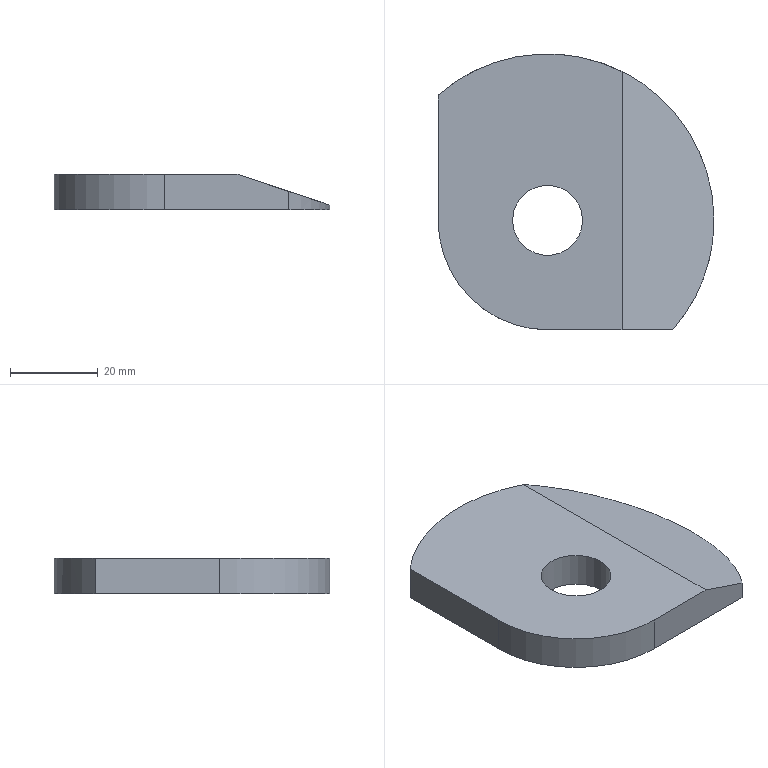Part | NX | features DATUM_CSYS 3, EXTRUDE 2, SKETCH 2 | 1 solid | 10 faces | box 62.986 x 63 x 8 mm | volume 22550 mm3 | plane 6 | cylinder 4 | commonest cylinder face diameters 76 x2 16 x1 50 x1
STEP:
#1=CARTESIAN_POINT('',(17.001,-24.999,8.));
#2=VERTEX_POINT('',#1);
#3=CARTESIAN_POINT('',(28.619,-24.999,4.125));
#4=VERTEX_POINT('',#3);
#5=CARTESIAN_POINT('',(1.895,-24.999,13.039));
#6=DIRECTION('',(0.9486,0.,-0.3164));
#7=VECTOR('',#6,1000.);
#8=LINE('',#5,#7);
#9=EDGE_CURVE('',#2,#4,#8,.T.);
#10=ORIENTED_EDGE('',*,*,#9,.F.);
#11=CARTESIAN_POINT('',(0.2147,-24.999,8.));
#12=VERTEX_POINT('',#11);
#13=CARTESIAN_POINT('',(0.2147,-24.999,8.));
#14=DIRECTION('',(1.,0.,0.));
#15=VECTOR('',#14,1000.);
#16=LINE('',#13,#15);
#17=EDGE_CURVE('',#12,#2,#16,.T.);
#18=ORIENTED_EDGE('',*,*,#17,.F.);
#19=CARTESIAN_POINT('',(0.2147,-24.999,0.));
#20=VERTEX_POINT('',#19);
#21=CARTESIAN_POINT('',(0.2147,-24.999,8.));
#22=DIRECTION('',(0.,0.,-1.));
#23=VECTOR('',#22,1000.);
#24=LINE('',#21,#23);
#25=EDGE_CURVE('',#12,#20,#24,.T.);
#26=ORIENTED_EDGE('',*,*,#25,.T.);
#27=CARTESIAN_POINT('',(28.619,-24.999,0.));
#28=VERTEX_POINT('',#27);
#29=CARTESIAN_POINT('',(0.2147,-24.999,0.));
#30=DIRECTION('',(1.,0.,0.));
#31=VECTOR('',#30,1000.);
#32=LINE('',#29,#31);
#33=EDGE_CURVE('',#20,#28,#32,.T.);
#34=ORIENTED_EDGE('',*,*,#33,.T.);
#35=CARTESIAN_POINT('',(28.619,-24.999,8.));
#36=DIRECTION('',(0.,0.,-1.));
#37=VECTOR('',#36,1000.);
#38=LINE('',#35,#37);
#39=EDGE_CURVE('',#4,#28,#38,.T.);
#40=ORIENTED_EDGE('',*,*,#39,.F.);
#41=EDGE_LOOP('',(#10,#18,#26,#34,#40));
#42=FACE_BOUND('',#41,.T.);
#43=CARTESIAN_POINT('',(0.2147,-24.999,8.));
#44=DIRECTION('',(0.,1.,0.));
#45=DIRECTION('',(-1.,0.,0.));
#46=AXIS2_PLACEMENT_3D('',#43,#44,#45);
#47=PLANE('',#46);
#48=ADVANCED_FACE('',(#42),#47,.F.);
#49=CARTESIAN_POINT('',(37.986,-1.014,1.));
#50=VERTEX_POINT('',#49);
#51=CARTESIAN_POINT('',(0.,0.,13.671));
#52=DIRECTION('',(0.3164,0.,0.9486));
#53=DIRECTION('',(0.9486,0.,-0.3164));
#54=AXIS2_PLACEMENT_3D('',#51,#52,#53);
#55=ELLIPSE('',#54,40.058,38.);
#56=EDGE_CURVE('',#4,#50,#55,.T.);
#57=ORIENTED_EDGE('',*,*,#56,.F.);
#58=ORIENTED_EDGE('',*,*,#39,.T.);
#59=CARTESIAN_POINT('',(37.986,-1.014,0.));
#60=VERTEX_POINT('',#59);
#61=CARTESIAN_POINT('',(0.,0.,0.));
#62=DIRECTION('',(0.,0.,1.));
#63=DIRECTION('',(1.,0.,0.));
#64=AXIS2_PLACEMENT_3D('',#61,#62,#63);
#65=CIRCLE('',#64,38.);
#66=EDGE_CURVE('',#28,#60,#65,.T.);
#67=ORIENTED_EDGE('',*,*,#66,.T.);
#68=CARTESIAN_POINT('',(37.986,-1.014,8.));
#69=DIRECTION('',(0.,0.,-1.));
#70=VECTOR('',#69,1000.);
#71=LINE('',#68,#70);
#72=EDGE_CURVE('',#50,#60,#71,.T.);
#73=ORIENTED_EDGE('',*,*,#72,.F.);
#74=EDGE_LOOP('',(#57,#58,#67,#73));
#75=FACE_BOUND('',#74,.T.);
#76=CARTESIAN_POINT('',(0.,0.,8.));
#77=DIRECTION('',(0.,0.,-1.));
#78=DIRECTION('',(-1.,0.,0.));
#79=AXIS2_PLACEMENT_3D('',#76,#77,#78);
#80=CYLINDRICAL_SURFACE('',#79,38.);
#81=ADVANCED_FACE('',(#75),#80,.T.);
#82=CARTESIAN_POINT('',(37.986,1.014,1.));
#83=VERTEX_POINT('',#82);
#84=CARTESIAN_POINT('',(17.001,33.985,8.));
#85=VERTEX_POINT('',#84);
#86=CARTESIAN_POINT('',(0.,0.,13.671));
#87=DIRECTION('',(0.3164,0.,0.9486));
#88=DIRECTION('',(0.9486,0.,-0.3164));
#89=AXIS2_PLACEMENT_3D('',#86,#87,#88);
#90=ELLIPSE('',#89,40.058,38.);
#91=EDGE_CURVE('',#83,#85,#90,.T.);
#92=ORIENTED_EDGE('',*,*,#91,.F.);
#93=CARTESIAN_POINT('',(37.986,1.014,0.));
#94=VERTEX_POINT('',#93);
#95=CARTESIAN_POINT('',(37.986,1.014,8.));
#96=DIRECTION('',(0.,0.,-1.));
#97=VECTOR('',#96,1000.);
#98=LINE('',#95,#97);
#99=EDGE_CURVE('',#94,#83,#98,.F.);
#100=ORIENTED_EDGE('',*,*,#99,.F.);
#101=CARTESIAN_POINT('',(-24.999,28.619,0.));
#102=VERTEX_POINT('',#101);
#103=CARTESIAN_POINT('',(0.,0.,0.));
#104=DIRECTION('',(0.,0.,1.));
#105=DIRECTION('',(1.,0.,0.));
#106=AXIS2_PLACEMENT_3D('',#103,#104,#105);
#107=CIRCLE('',#106,38.);
#108=EDGE_CURVE('',#94,#102,#107,.T.);
#109=ORIENTED_EDGE('',*,*,#108,.T.);
#110=CARTESIAN_POINT('',(-24.999,28.619,8.));
#111=VERTEX_POINT('',#110);
#112=CARTESIAN_POINT('',(-24.999,28.619,8.));
#113=CARTESIAN_POINT('',(-24.999,28.619,5.333));
#114=CARTESIAN_POINT('',(-24.999,28.619,2.667));
#115=CARTESIAN_POINT('',(-24.999,28.619,0.));
#116=B_SPLINE_CURVE_WITH_KNOTS('',3,(#112,#113,#114,#115),.UNSPECIFIED.,.F.,.F.,(4,4),(0.,1.),.UNSPECIFIED.);
#117=EDGE_CURVE('',#111,#102,#116,.T.);
#118=ORIENTED_EDGE('',*,*,#117,.F.);
#119=CARTESIAN_POINT('',(0.,0.,8.));
#120=DIRECTION('',(0.,0.,1.));
#121=DIRECTION('',(1.,0.,0.));
#122=AXIS2_PLACEMENT_3D('',#119,#120,#121);
#123=CIRCLE('',#122,38.);
#124=EDGE_CURVE('',#85,#111,#123,.T.);
#125=ORIENTED_EDGE('',*,*,#124,.F.);
#126=EDGE_LOOP('',(#92,#100,#109,#118,#125));
#127=FACE_BOUND('',#126,.T.);
#128=CARTESIAN_POINT('',(0.,0.,8.));
#129=DIRECTION('',(0.,0.,-1.));
#130=DIRECTION('',(-1.,0.,0.));
#131=AXIS2_PLACEMENT_3D('',#128,#129,#130);
#132=CYLINDRICAL_SURFACE('',#131,38.);
#133=ADVANCED_FACE('',(#127),#132,.T.);
#134=CARTESIAN_POINT('',(-24.999,0.1887,8.));
#135=VERTEX_POINT('',#134);
#136=CARTESIAN_POINT('',(0.,0.,8.));
#137=DIRECTION('',(0.,0.,1.));
#138=DIRECTION('',(1.,0.,0.));
#139=AXIS2_PLACEMENT_3D('',#136,#137,#138);
#140=CIRCLE('',#139,25.);
#141=EDGE_CURVE('',#135,#12,#140,.T.);
#142=ORIENTED_EDGE('',*,*,#141,.T.);
#143=ORIENTED_EDGE('',*,*,#17,.T.);
#144=CARTESIAN_POINT('',(17.001,-38.,8.));
#145=DIRECTION('',(0.,1.,0.));
#146=VECTOR('',#145,1000.);
#147=LINE('',#144,#146);
#148=EDGE_CURVE('',#2,#85,#147,.T.);
#149=ORIENTED_EDGE('',*,*,#148,.T.);
#150=ORIENTED_EDGE('',*,*,#124,.T.);
#151=CARTESIAN_POINT('',(-24.999,28.619,8.));
#152=DIRECTION('',(0.,-1.,0.));
#153=VECTOR('',#152,1000.);
#154=LINE('',#151,#153);
#155=EDGE_CURVE('',#111,#135,#154,.T.);
#156=ORIENTED_EDGE('',*,*,#155,.T.);
#157=EDGE_LOOP('',(#142,#143,#149,#150,#156));
#158=FACE_BOUND('',#157,.T.);
#159=CARTESIAN_POINT('',(8.,0.,8.));
#160=VERTEX_POINT('',#159);
#161=CARTESIAN_POINT('',(0.,0.,8.));
#162=DIRECTION('',(0.,0.,1.));
#163=DIRECTION('',(1.,0.,0.));
#164=AXIS2_PLACEMENT_3D('',#161,#162,#163);
#165=CIRCLE('',#164,8.);
#166=EDGE_CURVE('',#160,#160,#165,.T.);
#167=ORIENTED_EDGE('',*,*,#166,.F.);
#168=EDGE_LOOP('',(#167));
#169=FACE_BOUND('',#168,.T.);
#170=CARTESIAN_POINT('',(0.,0.,8.));
#171=DIRECTION('',(0.,0.,1.));
#172=DIRECTION('',(1.,0.,0.));
#173=AXIS2_PLACEMENT_3D('',#170,#171,#172);
#174=PLANE('',#173);
#175=ADVANCED_FACE('',(#158,#169),#174,.T.);
#176=CARTESIAN_POINT('',(8.,0.,0.));
#177=VERTEX_POINT('',#176);
#178=CARTESIAN_POINT('',(0.,0.,0.));
#179=DIRECTION('',(0.,0.,1.));
#180=DIRECTION('',(1.,0.,0.));
#181=AXIS2_PLACEMENT_3D('',#178,#179,#180);
#182=CIRCLE('',#181,8.);
#183=EDGE_CURVE('',#177,#177,#182,.T.);
#184=ORIENTED_EDGE('',*,*,#183,.T.);
#185=EDGE_LOOP('',(#184));
#186=FACE_BOUND('',#185,.T.);
#187=CARTESIAN_POINT('',(37.986,-38.,0.));
#188=DIRECTION('',(0.,1.,0.));
#189=VECTOR('',#188,1000.);
#190=LINE('',#187,#189);
#191=EDGE_CURVE('',#60,#94,#190,.T.);
#192=ORIENTED_EDGE('',*,*,#191,.F.);
#193=ORIENTED_EDGE('',*,*,#66,.F.);
#194=ORIENTED_EDGE('',*,*,#33,.F.);
#195=CARTESIAN_POINT('',(-24.999,0.1887,0.));
#196=VERTEX_POINT('',#195);
#197=CARTESIAN_POINT('',(0.,0.,0.));
#198=DIRECTION('',(0.,0.,1.));
#199=DIRECTION('',(1.,0.,0.));
#200=AXIS2_PLACEMENT_3D('',#197,#198,#199);
#201=CIRCLE('',#200,25.);
#202=EDGE_CURVE('',#196,#20,#201,.T.);
#203=ORIENTED_EDGE('',*,*,#202,.F.);
#204=CARTESIAN_POINT('',(-24.999,28.619,0.));
#205=DIRECTION('',(0.,1.,0.));
#206=VECTOR('',#205,1000.);
#207=LINE('',#204,#206);
#208=EDGE_CURVE('',#102,#196,#207,.F.);
#209=ORIENTED_EDGE('',*,*,#208,.F.);
#210=ORIENTED_EDGE('',*,*,#108,.F.);
#211=EDGE_LOOP('',(#192,#193,#194,#203,#209,#210));
#212=FACE_BOUND('',#211,.T.);
#213=CARTESIAN_POINT('',(0.,0.,0.));
#214=DIRECTION('',(0.,0.,1.));
#215=DIRECTION('',(1.,0.,0.));
#216=AXIS2_PLACEMENT_3D('',#213,#214,#215);
#217=PLANE('',#216);
#218=ADVANCED_FACE('',(#186,#212),#217,.F.);
#219=ORIENTED_EDGE('',*,*,#208,.T.);
#220=CARTESIAN_POINT('',(-24.999,0.1887,0.));
#221=CARTESIAN_POINT('',(-24.999,0.1887,2.667));
#222=CARTESIAN_POINT('',(-24.999,0.1887,5.333));
#223=CARTESIAN_POINT('',(-24.999,0.1887,8.));
#224=B_SPLINE_CURVE_WITH_KNOTS('',3,(#220,#221,#222,#223),.UNSPECIFIED.,.F.,.F.,(4,4),(0.,1.),.UNSPECIFIED.);
#225=EDGE_CURVE('',#135,#196,#224,.F.);
#226=ORIENTED_EDGE('',*,*,#225,.F.);
#227=ORIENTED_EDGE('',*,*,#155,.F.);
#228=ORIENTED_EDGE('',*,*,#117,.T.);
#229=EDGE_LOOP('',(#219,#226,#227,#228));
#230=FACE_BOUND('',#229,.T.);
#231=CARTESIAN_POINT('',(-24.999,28.619,8.));
#232=DIRECTION('',(1.,0.,0.));
#233=DIRECTION('',(0.,1.,0.));
#234=AXIS2_PLACEMENT_3D('',#231,#232,#233);
#235=PLANE('',#234);
#236=ADVANCED_FACE('',(#230),#235,.F.);
#237=ORIENTED_EDGE('',*,*,#141,.F.);
#238=ORIENTED_EDGE('',*,*,#225,.T.);
#239=ORIENTED_EDGE('',*,*,#202,.T.);
#240=ORIENTED_EDGE('',*,*,#25,.F.);
#241=EDGE_LOOP('',(#237,#238,#239,#240));
#242=FACE_BOUND('',#241,.T.);
#243=CARTESIAN_POINT('',(0.,0.,8.));
#244=DIRECTION('',(0.,0.,-1.));
#245=DIRECTION('',(-1.,0.,0.));
#246=AXIS2_PLACEMENT_3D('',#243,#244,#245);
#247=CYLINDRICAL_SURFACE('',#246,25.);
#248=ADVANCED_FACE('',(#242),#247,.T.);
#249=ORIENTED_EDGE('',*,*,#166,.T.);
#250=EDGE_LOOP('',(#249));
#251=FACE_BOUND('',#250,.T.);
#252=ORIENTED_EDGE('',*,*,#183,.F.);
#253=EDGE_LOOP('',(#252));
#254=FACE_BOUND('',#253,.T.);
#255=CARTESIAN_POINT('',(0.,0.,8.));
#256=DIRECTION('',(0.,0.,-1.));
#257=DIRECTION('',(-1.,0.,0.));
#258=AXIS2_PLACEMENT_3D('',#255,#256,#257);
#259=CYLINDRICAL_SURFACE('',#258,8.);
#260=ADVANCED_FACE('',(#251,#254),#259,.F.);
#261=ORIENTED_EDGE('',*,*,#9,.T.);
#262=ORIENTED_EDGE('',*,*,#56,.T.);
#263=CARTESIAN_POINT('',(37.986,-38.,1.));
#264=DIRECTION('',(0.,1.,0.));
#265=VECTOR('',#264,1000.);
#266=LINE('',#263,#265);
#267=EDGE_CURVE('',#83,#50,#266,.F.);
#268=ORIENTED_EDGE('',*,*,#267,.F.);
#269=ORIENTED_EDGE('',*,*,#91,.T.);
#270=ORIENTED_EDGE('',*,*,#148,.F.);
#271=EDGE_LOOP('',(#261,#262,#268,#269,#270));
#272=FACE_BOUND('',#271,.T.);
#273=CARTESIAN_POINT('',(17.001,-38.,8.));
#274=DIRECTION('',(0.3164,0.,0.9486));
#275=DIRECTION('',(0.9486,0.,-0.3164));
#276=AXIS2_PLACEMENT_3D('',#273,#274,#275);
#277=PLANE('',#276);
#278=ADVANCED_FACE('',(#272),#277,.T.);
#279=ORIENTED_EDGE('',*,*,#72,.T.);
#280=ORIENTED_EDGE('',*,*,#191,.T.);
#281=ORIENTED_EDGE('',*,*,#99,.T.);
#282=ORIENTED_EDGE('',*,*,#267,.T.);
#283=EDGE_LOOP('',(#279,#280,#281,#282));
#284=FACE_BOUND('',#283,.T.);
#285=CARTESIAN_POINT('',(37.986,-38.,1.));
#286=DIRECTION('',(1.,0.,0.));
#287=DIRECTION('',(0.,0.,-1.));
#288=AXIS2_PLACEMENT_3D('',#285,#286,#287);
#289=PLANE('',#288);
#290=ADVANCED_FACE('',(#284),#289,.T.);
#291=CLOSED_SHELL('',(#48,#81,#133,#175,#218,#236,#248,#260,#278,#290));
#292=MANIFOLD_SOLID_BREP('',#291);
#293=(LENGTH_UNIT()NAMED_UNIT(*)SI_UNIT(.MILLI.,.METRE.));
#294=UNCERTAINTY_MEASURE_WITH_UNIT(LENGTH_MEASURE(0.0508),#293,'','');
#295=(NAMED_UNIT(*)PLANE_ANGLE_UNIT()SI_UNIT($,.RADIAN.));
#296=(NAMED_UNIT(*)SI_UNIT($,.STERADIAN.)SOLID_ANGLE_UNIT());
#297=(GEOMETRIC_REPRESENTATION_CONTEXT(3)GLOBAL_UNCERTAINTY_ASSIGNED_CONTEXT((#294))GLOBAL_UNIT_ASSIGNED_CONTEXT((#293,#295,#296))REPRESENTATION_CONTEXT('',''));
#298=ADVANCED_BREP_SHAPE_REPRESENTATION('',(#292),#297);